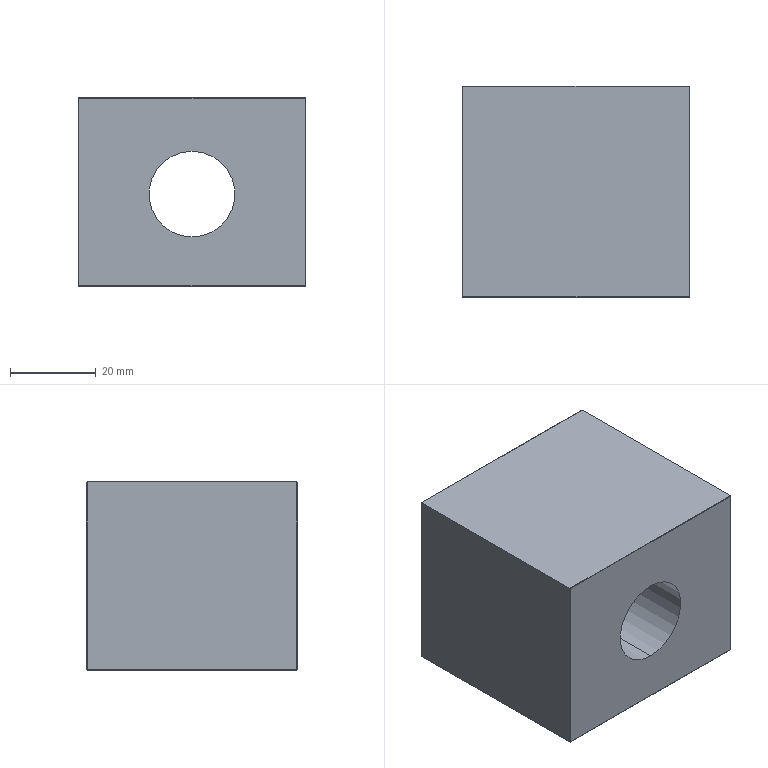Part | SolidWorks | features BaseBody 1 | 1 solid | 22 faces | box 53 x 49.2 x 44 mm | volume 99275 mm3 | plane 20 | cylinder 2 | commonest cylinder face diameters 20 x2
STEP:
#1=CARTESIAN_POINT('',(0.,24.6,9.5));
#2=VERTEX_POINT('',#1);
#3=CARTESIAN_POINT('',(0.,24.6,-10.5));
#4=VERTEX_POINT('',#3);
#5=CARTESIAN_POINT('',(0.,24.6,-0.5));
#6=DIRECTION('',(0.,-1.,0.));
#7=DIRECTION('',(0.,0.,-1.));
#8=AXIS2_PLACEMENT_3D('',#5,#6,#7);
#9=CIRCLE('',#8,10.);
#10=EDGE_CURVE('',#2,#4,#9,.T.);
#11=ORIENTED_EDGE('',*,*,#10,.F.);
#12=CARTESIAN_POINT('',(0.,-24.6,9.5));
#13=VERTEX_POINT('',#12);
#14=CARTESIAN_POINT('',(0.,24.6,9.5));
#15=DIRECTION('',(0.,-1.,0.));
#16=VECTOR('',#15,1000.);
#17=LINE('',#14,#16);
#18=EDGE_CURVE('',#2,#13,#17,.T.);
#19=ORIENTED_EDGE('',*,*,#18,.T.);
#20=CARTESIAN_POINT('',(0.,-24.6,-10.5));
#21=VERTEX_POINT('',#20);
#22=CARTESIAN_POINT('',(0.,-24.6,-0.5));
#23=DIRECTION('',(0.,1.,0.));
#24=DIRECTION('',(0.,0.,-1.));
#25=AXIS2_PLACEMENT_3D('',#22,#23,#24);
#26=CIRCLE('',#25,10.);
#27=EDGE_CURVE('',#21,#13,#26,.T.);
#28=ORIENTED_EDGE('',*,*,#27,.F.);
#29=CARTESIAN_POINT('',(0.,24.6,-10.5));
#30=DIRECTION('',(0.,-1.,0.));
#31=VECTOR('',#30,1000.);
#32=LINE('',#29,#31);
#33=EDGE_CURVE('',#4,#21,#32,.T.);
#34=ORIENTED_EDGE('',*,*,#33,.F.);
#35=EDGE_LOOP('',(#11,#19,#28,#34));
#36=FACE_OUTER_BOUND('',#35,.T.);
#37=CARTESIAN_POINT('',(0.,24.6,-0.5));
#38=DIRECTION('',(0.,-1.,0.));
#39=DIRECTION('',(0.,0.,-1.));
#40=AXIS2_PLACEMENT_3D('',#37,#38,#39);
#41=CYLINDRICAL_SURFACE('',#40,10.);
#42=ADVANCED_FACE('',(#36),#41,.F.);
#43=ORIENTED_EDGE('',*,*,#18,.F.);
#44=CARTESIAN_POINT('',(0.,24.6,-0.5));
#45=DIRECTION('',(0.,-1.,0.));
#46=DIRECTION('',(0.,0.,-1.));
#47=AXIS2_PLACEMENT_3D('',#44,#45,#46);
#48=CIRCLE('',#47,10.);
#49=EDGE_CURVE('',#4,#2,#48,.T.);
#50=ORIENTED_EDGE('',*,*,#49,.F.);
#51=ORIENTED_EDGE('',*,*,#33,.T.);
#52=CARTESIAN_POINT('',(0.,-24.6,-0.5));
#53=DIRECTION('',(0.,1.,0.));
#54=DIRECTION('',(0.,0.,-1.));
#55=AXIS2_PLACEMENT_3D('',#52,#53,#54);
#56=CIRCLE('',#55,10.);
#57=EDGE_CURVE('',#13,#21,#56,.T.);
#58=ORIENTED_EDGE('',*,*,#57,.F.);
#59=EDGE_LOOP('',(#43,#50,#51,#58));
#60=FACE_OUTER_BOUND('',#59,.T.);
#61=CARTESIAN_POINT('',(0.,24.6,-0.5));
#62=DIRECTION('',(0.,-1.,0.));
#63=DIRECTION('',(0.,0.,-1.));
#64=AXIS2_PLACEMENT_3D('',#61,#62,#63);
#65=CYLINDRICAL_SURFACE('',#64,10.);
#66=ADVANCED_FACE('',(#60),#65,.F.);
#67=CARTESIAN_POINT('',(-26.4,-24.6,21.9));
#68=VERTEX_POINT('',#67);
#69=CARTESIAN_POINT('',(-26.4,-24.6,-21.9));
#70=VERTEX_POINT('',#69);
#71=CARTESIAN_POINT('',(-26.4,-24.6,0.));
#72=DIRECTION('',(0.,0.,-1.));
#73=VECTOR('',#72,1000.);
#74=LINE('',#71,#73);
#75=EDGE_CURVE('',#68,#70,#74,.T.);
#76=ORIENTED_EDGE('',*,*,#75,.T.);
#77=CARTESIAN_POINT('',(26.4,-24.6,-21.9));
#78=VERTEX_POINT('',#77);
#79=CARTESIAN_POINT('',(0.,-24.6,-21.9));
#80=DIRECTION('',(1.,0.,0.));
#81=VECTOR('',#80,1000.);
#82=LINE('',#79,#81);
#83=EDGE_CURVE('',#70,#78,#82,.T.);
#84=ORIENTED_EDGE('',*,*,#83,.T.);
#85=CARTESIAN_POINT('',(26.4,-24.6,21.9));
#86=VERTEX_POINT('',#85);
#87=CARTESIAN_POINT('',(26.4,-24.6,0.));
#88=DIRECTION('',(0.,0.,1.));
#89=VECTOR('',#88,1000.);
#90=LINE('',#87,#89);
#91=EDGE_CURVE('',#78,#86,#90,.T.);
#92=ORIENTED_EDGE('',*,*,#91,.T.);
#93=CARTESIAN_POINT('',(0.,-24.6,21.9));
#94=DIRECTION('',(-1.,0.,0.));
#95=VECTOR('',#94,1000.);
#96=LINE('',#93,#95);
#97=EDGE_CURVE('',#86,#68,#96,.T.);
#98=ORIENTED_EDGE('',*,*,#97,.T.);
#99=EDGE_LOOP('',(#76,#84,#92,#98));
#100=FACE_OUTER_BOUND('',#99,.T.);
#101=ORIENTED_EDGE('',*,*,#27,.T.);
#102=ORIENTED_EDGE('',*,*,#57,.T.);
#103=EDGE_LOOP('',(#101,#102));
#104=FACE_BOUND('',#103,.T.);
#105=CARTESIAN_POINT('',(0.,-24.6,0.));
#106=DIRECTION('',(0.,-1.,0.));
#107=DIRECTION('',(0.,0.,-1.));
#108=AXIS2_PLACEMENT_3D('',#105,#106,#107);
#109=PLANE('',#108);
#110=ADVANCED_FACE('',(#100,#104),#109,.T.);
#111=CARTESIAN_POINT('',(-26.4,24.6,21.9));
#112=VERTEX_POINT('',#111);
#113=CARTESIAN_POINT('',(-26.4,24.6,-21.9));
#114=VERTEX_POINT('',#113);
#115=CARTESIAN_POINT('',(-26.4,24.6,0.));
#116=DIRECTION('',(0.,0.,-1.));
#117=VECTOR('',#116,1000.);
#118=LINE('',#115,#117);
#119=EDGE_CURVE('',#112,#114,#118,.T.);
#120=ORIENTED_EDGE('',*,*,#119,.F.);
#121=CARTESIAN_POINT('',(26.4,24.6,21.9));
#122=VERTEX_POINT('',#121);
#123=CARTESIAN_POINT('',(0.,24.6,21.9));
#124=DIRECTION('',(-1.,0.,0.));
#125=VECTOR('',#124,1000.);
#126=LINE('',#123,#125);
#127=EDGE_CURVE('',#122,#112,#126,.T.);
#128=ORIENTED_EDGE('',*,*,#127,.F.);
#129=CARTESIAN_POINT('',(26.4,24.6,-21.9));
#130=VERTEX_POINT('',#129);
#131=CARTESIAN_POINT('',(26.4,24.6,0.));
#132=DIRECTION('',(0.,0.,1.));
#133=VECTOR('',#132,1000.);
#134=LINE('',#131,#133);
#135=EDGE_CURVE('',#130,#122,#134,.T.);
#136=ORIENTED_EDGE('',*,*,#135,.F.);
#137=CARTESIAN_POINT('',(0.,24.6,-21.9));
#138=DIRECTION('',(1.,0.,0.));
#139=VECTOR('',#138,1000.);
#140=LINE('',#137,#139);
#141=EDGE_CURVE('',#114,#130,#140,.T.);
#142=ORIENTED_EDGE('',*,*,#141,.F.);
#143=EDGE_LOOP('',(#120,#128,#136,#142));
#144=FACE_OUTER_BOUND('',#143,.T.);
#145=ORIENTED_EDGE('',*,*,#49,.T.);
#146=ORIENTED_EDGE('',*,*,#10,.T.);
#147=EDGE_LOOP('',(#145,#146));
#148=FACE_BOUND('',#147,.T.);
#149=CARTESIAN_POINT('',(0.,24.6,0.));
#150=DIRECTION('',(0.,-1.,0.));
#151=DIRECTION('',(0.,0.,-1.));
#152=AXIS2_PLACEMENT_3D('',#149,#150,#151);
#153=PLANE('',#152);
#154=ADVANCED_FACE('',(#144,#148),#153,.F.);
#155=CARTESIAN_POINT('',(26.4,-24.5,-22.));
#156=VERTEX_POINT('',#155);
#157=CARTESIAN_POINT('',(26.4,-24.5,-22.));
#158=DIRECTION('',(0.,-0.7071,0.7071));
#159=VECTOR('',#158,1000.);
#160=LINE('',#157,#159);
#161=EDGE_CURVE('',#156,#78,#160,.T.);
#162=ORIENTED_EDGE('',*,*,#161,.T.);
#163=ORIENTED_EDGE('',*,*,#83,.F.);
#164=CARTESIAN_POINT('',(-26.4,-24.5,-22.));
#165=VERTEX_POINT('',#164);
#166=CARTESIAN_POINT('',(-26.4,-24.5,-22.));
#167=DIRECTION('',(0.,0.7071,-0.7071));
#168=VECTOR('',#167,1000.);
#169=LINE('',#166,#168);
#170=EDGE_CURVE('',#70,#165,#169,.T.);
#171=ORIENTED_EDGE('',*,*,#170,.T.);
#172=CARTESIAN_POINT('',(26.5,-24.5,-22.));
#173=DIRECTION('',(1.,0.,0.));
#174=VECTOR('',#173,1000.);
#175=LINE('',#172,#174);
#176=EDGE_CURVE('',#165,#156,#175,.T.);
#177=ORIENTED_EDGE('',*,*,#176,.T.);
#178=EDGE_LOOP('',(#162,#163,#171,#177));
#179=FACE_OUTER_BOUND('',#178,.T.);
#180=CARTESIAN_POINT('',(26.5,-24.5,-22.));
#181=DIRECTION('',(0.,-0.7071,-0.7071));
#182=DIRECTION('',(0.,0.7071,-0.7071));
#183=AXIS2_PLACEMENT_3D('',#180,#181,#182);
#184=PLANE('',#183);
#185=ADVANCED_FACE('',(#179),#184,.T.);
#186=CARTESIAN_POINT('',(-26.5,-24.5,22.));
#187=VERTEX_POINT('',#186);
#188=CARTESIAN_POINT('',(-26.4,-24.6,21.9));
#189=DIRECTION('',(-0.5774,0.5774,0.5774));
#190=VECTOR('',#189,1000.);
#191=LINE('',#188,#190);
#192=EDGE_CURVE('',#68,#187,#191,.T.);
#193=ORIENTED_EDGE('',*,*,#192,.T.);
#194=CARTESIAN_POINT('',(-26.5,-24.5,-21.9));
#195=VERTEX_POINT('',#194);
#196=CARTESIAN_POINT('',(-26.5,-24.5,-22.));
#197=DIRECTION('',(0.,0.,-1.));
#198=VECTOR('',#197,1000.);
#199=LINE('',#196,#198);
#200=EDGE_CURVE('',#187,#195,#199,.T.);
#201=ORIENTED_EDGE('',*,*,#200,.T.);
#202=CARTESIAN_POINT('',(-26.5,-24.5,-21.9));
#203=DIRECTION('',(0.7071,-0.7071,0.));
#204=VECTOR('',#203,1000.);
#205=LINE('',#202,#204);
#206=EDGE_CURVE('',#195,#70,#205,.T.);
#207=ORIENTED_EDGE('',*,*,#206,.T.);
#208=ORIENTED_EDGE('',*,*,#75,.F.);
#209=EDGE_LOOP('',(#193,#201,#207,#208));
#210=FACE_OUTER_BOUND('',#209,.T.);
#211=CARTESIAN_POINT('',(-26.5,-24.5,-22.));
#212=DIRECTION('',(-0.7071,-0.7071,0.));
#213=DIRECTION('',(0.7071,-0.7071,0.));
#214=AXIS2_PLACEMENT_3D('',#211,#212,#213);
#215=PLANE('',#214);
#216=ADVANCED_FACE('',(#210),#215,.T.);
#217=CARTESIAN_POINT('',(26.5,-24.5,22.));
#218=VERTEX_POINT('',#217);
#219=CARTESIAN_POINT('',(26.4,-24.6,21.9));
#220=DIRECTION('',(0.5774,0.5774,0.5774));
#221=VECTOR('',#220,1000.);
#222=LINE('',#219,#221);
#223=EDGE_CURVE('',#86,#218,#222,.T.);
#224=ORIENTED_EDGE('',*,*,#223,.T.);
#225=CARTESIAN_POINT('',(26.5,-24.5,22.));
#226=DIRECTION('',(-1.,0.,0.));
#227=VECTOR('',#226,1000.);
#228=LINE('',#225,#227);
#229=EDGE_CURVE('',#218,#187,#228,.T.);
#230=ORIENTED_EDGE('',*,*,#229,.T.);
#231=ORIENTED_EDGE('',*,*,#192,.F.);
#232=ORIENTED_EDGE('',*,*,#97,.F.);
#233=EDGE_LOOP('',(#224,#230,#231,#232));
#234=FACE_OUTER_BOUND('',#233,.T.);
#235=CARTESIAN_POINT('',(26.5,-24.5,22.));
#236=DIRECTION('',(0.,-0.7071,0.7071));
#237=DIRECTION('',(0.,-0.7071,-0.7071));
#238=AXIS2_PLACEMENT_3D('',#235,#236,#237);
#239=PLANE('',#238);
#240=ADVANCED_FACE('',(#234),#239,.T.);
#241=ORIENTED_EDGE('',*,*,#223,.F.);
#242=ORIENTED_EDGE('',*,*,#91,.F.);
#243=CARTESIAN_POINT('',(26.5,-24.5,-21.9));
#244=VERTEX_POINT('',#243);
#245=CARTESIAN_POINT('',(26.5,-24.5,-21.9));
#246=DIRECTION('',(0.7071,0.7071,0.));
#247=VECTOR('',#246,1000.);
#248=LINE('',#245,#247);
#249=EDGE_CURVE('',#78,#244,#248,.T.);
#250=ORIENTED_EDGE('',*,*,#249,.T.);
#251=CARTESIAN_POINT('',(26.5,-24.5,-22.));
#252=DIRECTION('',(0.,0.,1.));
#253=VECTOR('',#252,1000.);
#254=LINE('',#251,#253);
#255=EDGE_CURVE('',#244,#218,#254,.T.);
#256=ORIENTED_EDGE('',*,*,#255,.T.);
#257=EDGE_LOOP('',(#241,#242,#250,#256));
#258=FACE_OUTER_BOUND('',#257,.T.);
#259=CARTESIAN_POINT('',(26.5,-24.5,-22.));
#260=DIRECTION('',(0.7071,-0.7071,0.));
#261=DIRECTION('',(0.7071,0.7071,0.));
#262=AXIS2_PLACEMENT_3D('',#259,#260,#261);
#263=PLANE('',#262);
#264=ADVANCED_FACE('',(#258),#263,.T.);
#265=ORIENTED_EDGE('',*,*,#141,.T.);
#266=CARTESIAN_POINT('',(26.4,24.5,-22.));
#267=VERTEX_POINT('',#266);
#268=CARTESIAN_POINT('',(26.4,24.6,-21.9));
#269=DIRECTION('',(0.,0.7071,0.7071));
#270=VECTOR('',#269,1000.);
#271=LINE('',#268,#270);
#272=EDGE_CURVE('',#267,#130,#271,.T.);
#273=ORIENTED_EDGE('',*,*,#272,.F.);
#274=CARTESIAN_POINT('',(-26.4,24.5,-22.));
#275=VERTEX_POINT('',#274);
#276=CARTESIAN_POINT('',(0.,24.5,-22.));
#277=DIRECTION('',(1.,0.,0.));
#278=VECTOR('',#277,1000.);
#279=LINE('',#276,#278);
#280=EDGE_CURVE('',#275,#267,#279,.T.);
#281=ORIENTED_EDGE('',*,*,#280,.F.);
#282=CARTESIAN_POINT('',(-26.4,24.6,-21.9));
#283=DIRECTION('',(0.,-0.7071,-0.7071));
#284=VECTOR('',#283,1000.);
#285=LINE('',#282,#284);
#286=EDGE_CURVE('',#114,#275,#285,.T.);
#287=ORIENTED_EDGE('',*,*,#286,.F.);
#288=EDGE_LOOP('',(#265,#273,#281,#287));
#289=FACE_OUTER_BOUND('',#288,.T.);
#290=CARTESIAN_POINT('',(0.,24.6,-21.9));
#291=DIRECTION('',(0.,-0.7071,0.7071));
#292=DIRECTION('',(0.,-0.7071,-0.7071));
#293=AXIS2_PLACEMENT_3D('',#290,#291,#292);
#294=PLANE('',#293);
#295=ADVANCED_FACE('',(#289),#294,.F.);
#296=ORIENTED_EDGE('',*,*,#119,.T.);
#297=CARTESIAN_POINT('',(-26.5,24.5,-21.9));
#298=VERTEX_POINT('',#297);
#299=CARTESIAN_POINT('',(-26.4,24.6,-21.9));
#300=DIRECTION('',(0.7071,0.7071,0.));
#301=VECTOR('',#300,1000.);
#302=LINE('',#299,#301);
#303=EDGE_CURVE('',#298,#114,#302,.T.);
#304=ORIENTED_EDGE('',*,*,#303,.F.);
#305=CARTESIAN_POINT('',(-26.5,24.5,22.));
#306=VERTEX_POINT('',#305);
#307=CARTESIAN_POINT('',(-26.5,24.5,0.));
#308=DIRECTION('',(0.,0.,-1.));
#309=VECTOR('',#308,1000.);
#310=LINE('',#307,#309);
#311=EDGE_CURVE('',#306,#298,#310,.T.);
#312=ORIENTED_EDGE('',*,*,#311,.F.);
#313=CARTESIAN_POINT('',(-26.4,24.6,21.9));
#314=DIRECTION('',(-0.5774,-0.5774,0.5774));
#315=VECTOR('',#314,1000.);
#316=LINE('',#313,#315);
#317=EDGE_CURVE('',#112,#306,#316,.T.);
#318=ORIENTED_EDGE('',*,*,#317,.F.);
#319=EDGE_LOOP('',(#296,#304,#312,#318));
#320=FACE_OUTER_BOUND('',#319,.T.);
#321=CARTESIAN_POINT('',(-26.4,24.6,0.));
#322=DIRECTION('',(0.7071,-0.7071,0.));
#323=DIRECTION('',(0.7071,0.7071,0.));
#324=AXIS2_PLACEMENT_3D('',#321,#322,#323);
#325=PLANE('',#324);
#326=ADVANCED_FACE('',(#320),#325,.F.);
#327=ORIENTED_EDGE('',*,*,#127,.T.);
#328=ORIENTED_EDGE('',*,*,#317,.T.);
#329=CARTESIAN_POINT('',(26.5,24.5,22.));
#330=VERTEX_POINT('',#329);
#331=CARTESIAN_POINT('',(0.,24.5,22.));
#332=DIRECTION('',(-1.,0.,0.));
#333=VECTOR('',#332,1000.);
#334=LINE('',#331,#333);
#335=EDGE_CURVE('',#330,#306,#334,.T.);
#336=ORIENTED_EDGE('',*,*,#335,.F.);
#337=CARTESIAN_POINT('',(26.4,24.6,21.9));
#338=DIRECTION('',(0.5774,-0.5774,0.5774));
#339=VECTOR('',#338,1000.);
#340=LINE('',#337,#339);
#341=EDGE_CURVE('',#122,#330,#340,.T.);
#342=ORIENTED_EDGE('',*,*,#341,.F.);
#343=EDGE_LOOP('',(#327,#328,#336,#342));
#344=FACE_OUTER_BOUND('',#343,.T.);
#345=CARTESIAN_POINT('',(0.,24.6,21.9));
#346=DIRECTION('',(0.,-0.7071,-0.7071));
#347=DIRECTION('',(0.,0.7071,-0.7071));
#348=AXIS2_PLACEMENT_3D('',#345,#346,#347);
#349=PLANE('',#348);
#350=ADVANCED_FACE('',(#344),#349,.F.);
#351=CARTESIAN_POINT('',(26.5,24.5,-21.9));
#352=VERTEX_POINT('',#351);
#353=CARTESIAN_POINT('',(26.5,24.5,0.));
#354=DIRECTION('',(0.,0.,1.));
#355=VECTOR('',#354,1000.);
#356=LINE('',#353,#355);
#357=EDGE_CURVE('',#352,#330,#356,.T.);
#358=ORIENTED_EDGE('',*,*,#357,.F.);
#359=CARTESIAN_POINT('',(26.4,24.6,-21.9));
#360=DIRECTION('',(0.7071,-0.7071,0.));
#361=VECTOR('',#360,1000.);
#362=LINE('',#359,#361);
#363=EDGE_CURVE('',#130,#352,#362,.T.);
#364=ORIENTED_EDGE('',*,*,#363,.F.);
#365=ORIENTED_EDGE('',*,*,#135,.T.);
#366=ORIENTED_EDGE('',*,*,#341,.T.);
#367=EDGE_LOOP('',(#358,#364,#365,#366));
#368=FACE_OUTER_BOUND('',#367,.T.);
#369=CARTESIAN_POINT('',(26.4,24.6,0.));
#370=DIRECTION('',(-0.7071,-0.7071,0.));
#371=DIRECTION('',(0.7071,-0.7071,0.));
#372=AXIS2_PLACEMENT_3D('',#369,#370,#371);
#373=PLANE('',#372);
#374=ADVANCED_FACE('',(#368),#373,.F.);
#375=CARTESIAN_POINT('',(26.4,-24.5,-22.));
#376=DIRECTION('',(0.7071,0.,0.7071));
#377=VECTOR('',#376,1000.);
#378=LINE('',#375,#377);
#379=EDGE_CURVE('',#156,#244,#378,.T.);
#380=ORIENTED_EDGE('',*,*,#379,.T.);
#381=ORIENTED_EDGE('',*,*,#249,.F.);
#382=ORIENTED_EDGE('',*,*,#161,.F.);
#383=EDGE_LOOP('',(#380,#381,#382));
#384=FACE_OUTER_BOUND('',#383,.T.);
#385=CARTESIAN_POINT('',(26.5,-24.5,-21.9));
#386=DIRECTION('',(0.5774,-0.5774,-0.5774));
#387=DIRECTION('',(-0.7071,0.,-0.7071));
#388=AXIS2_PLACEMENT_3D('',#385,#386,#387);
#389=PLANE('',#388);
#390=ADVANCED_FACE('',(#384),#389,.T.);
#391=ORIENTED_EDGE('',*,*,#176,.F.);
#392=CARTESIAN_POINT('',(-26.4,24.6,-22.));
#393=DIRECTION('',(0.,-1.,0.));
#394=VECTOR('',#393,1000.);
#395=LINE('',#392,#394);
#396=EDGE_CURVE('',#275,#165,#395,.T.);
#397=ORIENTED_EDGE('',*,*,#396,.F.);
#398=ORIENTED_EDGE('',*,*,#280,.T.);
#399=CARTESIAN_POINT('',(26.4,24.6,-22.));
#400=DIRECTION('',(0.,1.,0.));
#401=VECTOR('',#400,1000.);
#402=LINE('',#399,#401);
#403=EDGE_CURVE('',#156,#267,#402,.T.);
#404=ORIENTED_EDGE('',*,*,#403,.F.);
#405=EDGE_LOOP('',(#391,#397,#398,#404));
#406=FACE_OUTER_BOUND('',#405,.T.);
#407=CARTESIAN_POINT('',(26.5,24.6,-22.));
#408=DIRECTION('',(0.,0.,1.));
#409=DIRECTION('',(1.,0.,0.));
#410=AXIS2_PLACEMENT_3D('',#407,#408,#409);
#411=PLANE('',#410);
#412=ADVANCED_FACE('',(#406),#411,.F.);
#413=ORIENTED_EDGE('',*,*,#170,.F.);
#414=ORIENTED_EDGE('',*,*,#206,.F.);
#415=CARTESIAN_POINT('',(-26.4,-24.5,-22.));
#416=DIRECTION('',(0.7071,0.,-0.7071));
#417=VECTOR('',#416,1000.);
#418=LINE('',#415,#417);
#419=EDGE_CURVE('',#195,#165,#418,.T.);
#420=ORIENTED_EDGE('',*,*,#419,.T.);
#421=EDGE_LOOP('',(#413,#414,#420));
#422=FACE_OUTER_BOUND('',#421,.T.);
#423=CARTESIAN_POINT('',(-26.4,-24.5,-22.));
#424=DIRECTION('',(-0.5774,-0.5774,-0.5774));
#425=DIRECTION('',(-0.7071,0.,0.7071));
#426=AXIS2_PLACEMENT_3D('',#423,#424,#425);
#427=PLANE('',#426);
#428=ADVANCED_FACE('',(#422),#427,.T.);
#429=ORIENTED_EDGE('',*,*,#200,.F.);
#430=CARTESIAN_POINT('',(-26.5,24.6,22.));
#431=DIRECTION('',(0.,-1.,0.));
#432=VECTOR('',#431,1000.);
#433=LINE('',#430,#432);
#434=EDGE_CURVE('',#306,#187,#433,.T.);
#435=ORIENTED_EDGE('',*,*,#434,.F.);
#436=ORIENTED_EDGE('',*,*,#311,.T.);
#437=CARTESIAN_POINT('',(-26.5,24.6,-21.9));
#438=DIRECTION('',(0.,1.,0.));
#439=VECTOR('',#438,1000.);
#440=LINE('',#437,#439);
#441=EDGE_CURVE('',#195,#298,#440,.T.);
#442=ORIENTED_EDGE('',*,*,#441,.F.);
#443=EDGE_LOOP('',(#429,#435,#436,#442));
#444=FACE_OUTER_BOUND('',#443,.T.);
#445=CARTESIAN_POINT('',(-26.5,24.6,-22.));
#446=DIRECTION('',(1.,0.,0.));
#447=DIRECTION('',(0.,0.,-1.));
#448=AXIS2_PLACEMENT_3D('',#445,#446,#447);
#449=PLANE('',#448);
#450=ADVANCED_FACE('',(#444),#449,.F.);
#451=ORIENTED_EDGE('',*,*,#229,.F.);
#452=CARTESIAN_POINT('',(26.5,24.6,22.));
#453=DIRECTION('',(0.,-1.,0.));
#454=VECTOR('',#453,1000.);
#455=LINE('',#452,#454);
#456=EDGE_CURVE('',#330,#218,#455,.T.);
#457=ORIENTED_EDGE('',*,*,#456,.F.);
#458=ORIENTED_EDGE('',*,*,#335,.T.);
#459=ORIENTED_EDGE('',*,*,#434,.T.);
#460=EDGE_LOOP('',(#451,#457,#458,#459));
#461=FACE_OUTER_BOUND('',#460,.T.);
#462=CARTESIAN_POINT('',(26.5,24.6,22.));
#463=DIRECTION('',(0.,0.,-1.));
#464=DIRECTION('',(-1.,0.,0.));
#465=AXIS2_PLACEMENT_3D('',#462,#463,#464);
#466=PLANE('',#465);
#467=ADVANCED_FACE('',(#461),#466,.F.);
#468=ORIENTED_EDGE('',*,*,#255,.F.);
#469=CARTESIAN_POINT('',(26.5,24.6,-21.9));
#470=DIRECTION('',(0.,-1.,0.));
#471=VECTOR('',#470,1000.);
#472=LINE('',#469,#471);
#473=EDGE_CURVE('',#352,#244,#472,.T.);
#474=ORIENTED_EDGE('',*,*,#473,.F.);
#475=ORIENTED_EDGE('',*,*,#357,.T.);
#476=ORIENTED_EDGE('',*,*,#456,.T.);
#477=EDGE_LOOP('',(#468,#474,#475,#476));
#478=FACE_OUTER_BOUND('',#477,.T.);
#479=CARTESIAN_POINT('',(26.5,24.6,-22.));
#480=DIRECTION('',(-1.,0.,0.));
#481=DIRECTION('',(0.,0.,1.));
#482=AXIS2_PLACEMENT_3D('',#479,#480,#481);
#483=PLANE('',#482);
#484=ADVANCED_FACE('',(#478),#483,.F.);
#485=ORIENTED_EDGE('',*,*,#286,.T.);
#486=CARTESIAN_POINT('',(-26.4,24.5,-22.));
#487=DIRECTION('',(-0.7071,0.,0.7071));
#488=VECTOR('',#487,1000.);
#489=LINE('',#486,#488);
#490=EDGE_CURVE('',#275,#298,#489,.T.);
#491=ORIENTED_EDGE('',*,*,#490,.T.);
#492=ORIENTED_EDGE('',*,*,#303,.T.);
#493=EDGE_LOOP('',(#485,#491,#492));
#494=FACE_OUTER_BOUND('',#493,.T.);
#495=CARTESIAN_POINT('',(-26.4,24.5,-22.));
#496=DIRECTION('',(-0.5774,0.5774,-0.5774));
#497=DIRECTION('',(-0.7071,0.,0.7071));
#498=AXIS2_PLACEMENT_3D('',#495,#496,#497);
#499=PLANE('',#498);
#500=ADVANCED_FACE('',(#494),#499,.T.);
#501=ORIENTED_EDGE('',*,*,#363,.T.);
#502=CARTESIAN_POINT('',(26.4,24.5,-22.));
#503=DIRECTION('',(-0.7071,0.,-0.7071));
#504=VECTOR('',#503,1000.);
#505=LINE('',#502,#504);
#506=EDGE_CURVE('',#352,#267,#505,.T.);
#507=ORIENTED_EDGE('',*,*,#506,.T.);
#508=ORIENTED_EDGE('',*,*,#272,.T.);
#509=EDGE_LOOP('',(#501,#507,#508));
#510=FACE_OUTER_BOUND('',#509,.T.);
#511=CARTESIAN_POINT('',(26.4,24.5,-22.));
#512=DIRECTION('',(0.5774,0.5774,-0.5774));
#513=DIRECTION('',(-0.7071,0.,-0.7071));
#514=AXIS2_PLACEMENT_3D('',#511,#512,#513);
#515=PLANE('',#514);
#516=ADVANCED_FACE('',(#510),#515,.T.);
#517=ORIENTED_EDGE('',*,*,#473,.T.);
#518=ORIENTED_EDGE('',*,*,#379,.F.);
#519=ORIENTED_EDGE('',*,*,#403,.T.);
#520=ORIENTED_EDGE('',*,*,#506,.F.);
#521=EDGE_LOOP('',(#517,#518,#519,#520));
#522=FACE_OUTER_BOUND('',#521,.T.);
#523=CARTESIAN_POINT('',(26.4,24.6,-22.));
#524=DIRECTION('',(-0.7071,0.,0.7071));
#525=DIRECTION('',(0.7071,0.,0.7071));
#526=AXIS2_PLACEMENT_3D('',#523,#524,#525);
#527=PLANE('',#526);
#528=ADVANCED_FACE('',(#522),#527,.F.);
#529=ORIENTED_EDGE('',*,*,#396,.T.);
#530=ORIENTED_EDGE('',*,*,#419,.F.);
#531=ORIENTED_EDGE('',*,*,#441,.T.);
#532=ORIENTED_EDGE('',*,*,#490,.F.);
#533=EDGE_LOOP('',(#529,#530,#531,#532));
#534=FACE_OUTER_BOUND('',#533,.T.);
#535=CARTESIAN_POINT('',(-26.5,24.6,-21.9));
#536=DIRECTION('',(0.7071,0.,0.7071));
#537=DIRECTION('',(0.7071,0.,-0.7071));
#538=AXIS2_PLACEMENT_3D('',#535,#536,#537);
#539=PLANE('',#538);
#540=ADVANCED_FACE('',(#534),#539,.F.);
#541=CLOSED_SHELL('',(#42,#66,#110,#154,#185,#216,#240,#264,#295,#326,#350,#374,#390,#412,#428,#450,#467,#484,#500,#516,#528,#540));
#542=MANIFOLD_SOLID_BREP('',#541);
#543=CARTESIAN_POINT('',(0.,0.,0.));
#544=DIRECTION('',(0.,0.,1.));
#545=DIRECTION('',(1.,0.,0.));
#546=AXIS2_PLACEMENT_3D('',#543,#544,#545);
#547=(LENGTH_UNIT()NAMED_UNIT(*)SI_UNIT(.MILLI.,.METRE.));
#548=UNCERTAINTY_MEASURE_WITH_UNIT(LENGTH_MEASURE(0.00001),#547,'','');
#549=(NAMED_UNIT(*)PLANE_ANGLE_UNIT()SI_UNIT($,.RADIAN.));
#550=(NAMED_UNIT(*)SI_UNIT($,.STERADIAN.)SOLID_ANGLE_UNIT());
#551=(GEOMETRIC_REPRESENTATION_CONTEXT(3)GLOBAL_UNCERTAINTY_ASSIGNED_CONTEXT((#548))GLOBAL_UNIT_ASSIGNED_CONTEXT((#547,#549,#550))REPRESENTATION_CONTEXT('',''));
#552=ADVANCED_BREP_SHAPE_REPRESENTATION('',(#542,#546),#551);